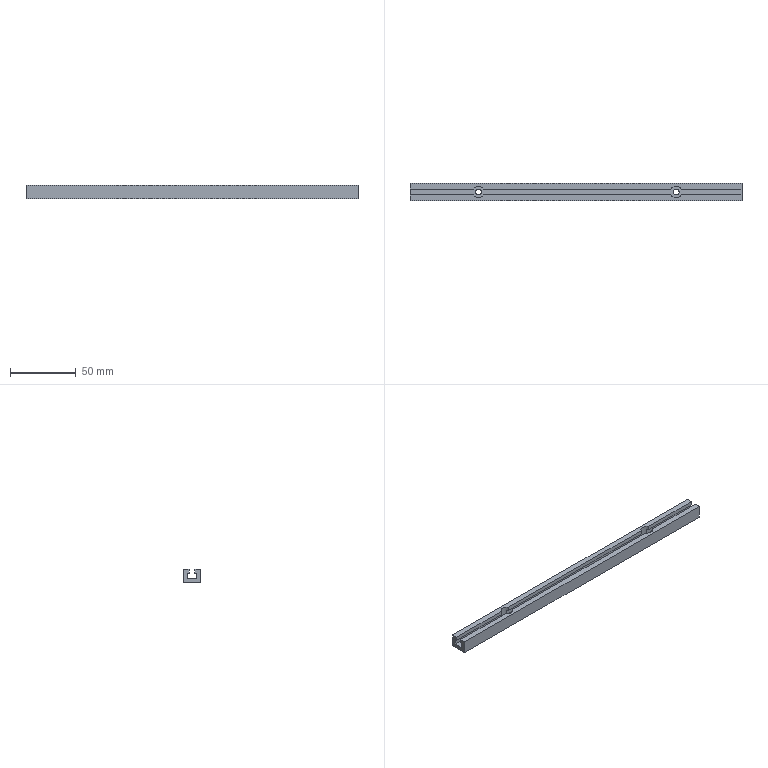Part | STEP file | Tube feed_id842_x_t | 1 solid | 32 faces | box 252 x 13 x 10 mm | volume 22066 mm3 | plane 26 | cylinder 6 | commonest cylinder face diameters 9 x4 4.5 x2